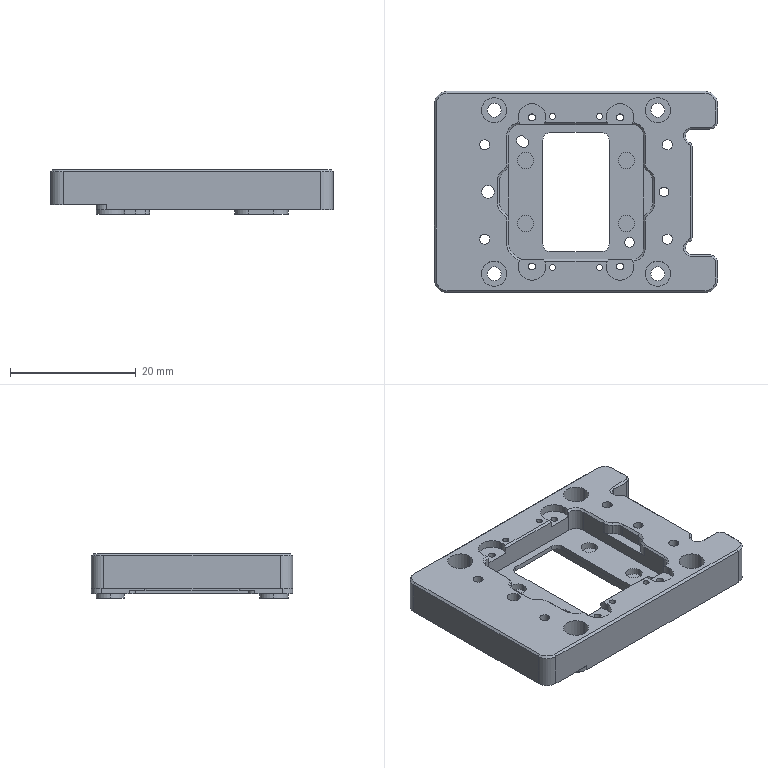NC program | NX | posted with a generic post | part box 45 x 32 x 7.05 mm
Lines 1920 to 2540 of 2540:
(PLANAR_MILL_COPY_COPY_COPY , TOOL : D6A45)
N3796 T01 M6
N3798 G54
N3800 G17 G0 G90 X13.45 Y12.567 S9500 M3
N3802 G43 Z30. H1
N3804 Z0.5
N3806 G94 G1 Z-0.5 F1250.
N3808 G3 X13.7 Y13. R0.5
N3810 X13. Y13.7 R0.7
N3812 X13.7 Y13. R-0.7
N3814 X13.45 Y13.433 R0.5
N3816 G1 Z0.5
N3818 G0 Z30.
N3820 X10.115 Y16.132
N3822 Z0.5
N3824 G1 Z-0.5
N3826 G3 X10.981 Y15.632 R1.
N3828 G1 X12.981
N3830 G2 X15.631 Y12.982 R2.65
N3832 X12.981 Y10.332 R2.65
N3834 G1 X8.981
N3836 G2 X7.064 Y11.153 R2.65
N3838 X7.096 Y11.735 R0.4
N3840 G3 X6.95 Y11.991 R0.15
N3842 G2 X6.432 Y12.259 R0.4
N3844 X8.981 Y15.632 R2.65
N3846 G1 X10.981
N3848 G3 X11.847 Y16.132 R1.
N3850 G1 Z0.5
N3852 G0 Z30.
N3854 X8.959 Y12.892
N3856 Z0.5
N3858 G1 Z-0.5
N3860 G3 X8.987 Y13.149 R0.5
N3862 X8.802 Y12.964 R0.185
N3864 X8.987 Y13.149 R-0.185
N3866 X9.014 Y12.892 R0.5
N3868 G1 Z0.5
N3870 G0 Z30.
N3872 X-12.567 Y13.45
N3874 Z0.5
N3876 G1 Z-0.5
N3878 G3 X-13. Y13.7 R0.5
N3880 X-13.7 Y13. R0.7
N3882 X-13. Y13.7 R-0.7
N3884 X-13.433 Y13.45 R0.5
N3886 G1 Z0.5
N3888 G0 Z30.
N3890 X-16.176 Y12.121
N3892 Z0.5
N3894 G1 Z-0.5
N3896 G3 X-15.676 Y12.987 R1.
N3898 G2 X-13.026 Y15.637 R2.65
N3900 X-15.676 Y12.987 R-2.65
N3902 G3 X-16.176 Y13.853 R1.
N3904 G1 Z0.5
N3906 G0 Z30.
N3908 X-13.433 Y-13.45
N3910 Z0.5
N3912 G1 Z-0.5
N3914 G3 X-13. Y-13.7 R0.5
N3916 X-12.3 Y-13. R0.7
N3918 X-13. Y-13.7 R-0.7
N3920 X-12.567 Y-13.45 R0.5
N3922 G1 Z0.5
N3924 G0 Z30.
N3926 X-10.159 Y-16.158
N3928 Z0.5
N3930 G1 Z-0.5
N3932 G3 X-11.025 Y-15.658 R1.
N3934 G1 X-13.025
N3936 G2 X-15.675 Y-13.008 R2.65
N3938 X-13.025 Y-10.358 R2.65
N3940 G1 X-9.025
N3942 G2 X-7.099 Y-11.187 R2.65
N3944 X-7.106 Y-11.744 R0.4
N3946 G3 X-6.963 Y-11.995 R0.15
N3948 G2 X-6.479 Y-12.272 R0.4
N3950 X-9.025 Y-15.658 R2.65
N3952 G1 X-11.025
N3954 G3 X-11.891 Y-16.158 R1.
N3956 G1 Z0.5
N3958 G0 Z30.
N3960 X-8.985 Y-12.956
N3962 Z0.5
N3964 G1 Z-0.5
N3966 G3 X-9.013 Y-13.213 R0.5
N3968 X-8.828 Y-13.028 R0.185
N3970 X-9.013 Y-13.213 R-0.185
N3972 X-9.04 Y-12.956 R0.5
N3974 G1 Z0.5
N3976 G0 Z30.
N3978 X13.842 Y-16.161
N3980 Z0.5
N3982 G1 Z-0.5
N3984 G3 X12.976 Y-15.661 R1.
N3986 G2 X10.326 Y-13.011 R2.65
N3988 X12.976 Y-15.661 R-2.65
N3990 G3 X12.11 Y-16.161 R1.
N3992 G1 Z0.5
N3994 G0 Z30.
N3996 X13.45 Y-13.433
N3998 Z0.5
N4000 G1 Z-0.5
N4002 G3 X13.7 Y-13. R0.5
N4004 X13. Y-12.3 R0.7
N4006 X13.7 Y-13. R-0.7
N4008 X13.45 Y-12.567 R0.5
N4010 G1 Z0.5
N4012 G0 Z30.
(PLANAR_MILL_COPY_COPY_COPY_COPY , TOOL : D6A45)
N4014 X-6.946 Y11.7
N4016 Z-0.2
N4018 G1 X-6.901 Z-0.212
N4020 X-6.85 Y11.751 Z-0.231
N4022 Y11.949 Z-0.285
N4024 X-6.901 Y12. Z-0.304
N4026 X-7.099 Z-0.357
N4028 X-7.15 Y11.949 Z-0.376
N4030 Y11.751 Z-0.43
N4032 X-7.099 Y11.7 Z-0.449
N4034 X-6.901 Z-0.502
N4036 X-6.85 Y11.751 Z-0.521
N4038 Y11.949 Z-0.575
N4040 X-6.901 Y12. Z-0.594
N4042 X-7.099 Z-0.647
N4044 X-7.15 Y11.949 Z-0.666
N4046 Y11.751 Z-0.719
N4048 X-7.099 Y11.7 Z-0.739
N4050 X-6.901 Z-0.792
N4052 X-6.85 Y11.751 Z-0.811
N4054 Y11.949 Z-0.864
N4056 X-6.901 Y12. Z-0.884
N4058 X-7.099 Z-0.937
N4060 X-7.15 Y11.949 Z-0.956
N4062 Y11.751 Z-1.009
N4064 X-7.099 Y11.7 Z-1.028
N4066 X-6.901 Z-1.082
N4068 X-6.85 Y11.751 Z-1.101
N4070 Y11.949 Z-1.154
N4072 X-6.901 Y12. Z-1.173
N4074 X-7. Z-1.2
N4076 G3 X-7.15 Y11.85 R0.15
N4078 X-7. Y12. R-0.15
N4080 X-6.891 Y11.765 R0.5
N4082 G1 Z-0.2
N4084 G0 Z30.
N4086 X-11.533 Y17.286
N4088 Z-0.2
N4090 G1 Z-1.2
N4092 Y17.268
N4094 G3 X-11.036 Y16.4 R1.
N4096 G1 X7.001
N4098 G3 X7.499 Y17.284 R1.
N4100 G1 Z-0.2
N4102 G0 Z30.
N4104 X11.433 Y-17.291
N4106 Z-0.2
N4108 G1 Z-1.2
N4110 Y-17.274
N4112 G3 X10.947 Y-16.4 R1.
N4114 G1 X-7.001
N4116 G3 X-7.488 Y-17.273 R1.
N4118 G1 X-14.561
N4120 G3 X-15.049 Y-16.4 R1.
N4122 G1 X-20.5
N4124 G2 X-22.9 Y-14. R2.4
N4126 G1 Y-11.214
N4128 G2 X-22.49 Y-10.224 R1.4
N4130 G1 X-22.276 Y-10.01
N4132 G2 X-21.286 Y-9.6 R1.4
N4134 G1 X-18.555
N4136 G3 X-19.552 Y-9.523 R1.
N4138 G1 Y-9.
N4140 Z-0.2
N4142 G0 Z30.
N4144 Y9.
N4146 Z-0.2
N4148 G1 Z-1.2
N4150 Y9.523
N4152 G3 X-18.555 Y9.6 R1.
N4154 G1 X-21.286
N4156 G2 X-22.276 Y10.01 R1.4
N4158 G1 X-22.49 Y10.224
N4160 G2 X-22.9 Y11.214 R1.4
N4162 G1 Y14.
N4164 G2 X-20.5 Y16.4 R2.4
N4166 G1 X-15.015
N4168 G3 X-14.518 Y17.286 R1.
N4170 G1 Z-0.2
N4172 G0 Z30.
N4174 X4.439 Y12.713
N4176 Z-0.2
N4178 G1 Z-1.2
N4180 X4.455 Y12.72
N4182 G3 X5.067 Y13.511 R1.
N4184 X4.25 Y13.8 R1.3
N4186 G1 X3.164
N4188 G2 X2.18 Y14.204 R1.4
N4190 G3 X-2.18 Y14.204 R3.1
N4192 G2 X-3.164 Y13.8 R1.4
N4194 G1 X-4.25
N4196 G3 X-5.55 Y12.5 R1.3
N4198 G1 Y-11.304
N4200 G3 X-4.679 Y-11.664 R1.
N4202 G1 X-4.503 Y-12.681
N4204 G3 X-5.103 Y-13.481 R1.
N4206 X-4.25 Y-13.8 R1.3
N4208 G1 X-3.164
N4210 G2 X-2.18 Y-14.204 R1.4
N4212 G3 X2.18 Y-14.204 R3.1
N4214 G2 X3.164 Y-13.8 R1.4
N4216 G1 X3.629
N4218 G3 X4.548 Y-13.419 R1.3
N4220 G1 X5.169 Y-12.798
N4222 G3 X5.55 Y-11.879 R1.3
N4224 G1 Y-10.917
N4226 G3 X4.668 Y-10.957 R1.
N4228 G1 Z-0.2
N4230 G0 Z30.
N4232 Y10.957
N4234 Z-0.2
N4236 G1 Z-1.2
N4238 G3 X5.55 Y10.917 R1.
N4240 G1 Y11.235
N4242 G3 X4.664 Y11.558 R1.
N4244 G1 Z-0.2
N4246 G0 Z30.
N4248 X-8.125 Y-7.876
N4250 Z-0.2
N4252 G1 Y-7.847 Z-0.208
N4254 X-8.226 Y-7.702 Z-0.255
N4256 X-8.369 Y-7.649 Z-0.296
N4258 X-8.226 Y-7.702 Z-0.337
N4260 X-8.125 Y-7.847 Z-0.384
N4262 Y-8.153 Z-0.466
N4264 X-8.347 Y-8.375 Z-0.55
N4266 X-8.522 Y-8.374 Z-0.597
N4268 X-8.347 Y-8.375 Z-0.644
N4270 X-8.125 Y-8.153 Z-0.728
N4272 Y-7.847 Z-0.81
N4274 X-8.226 Y-7.702 Z-0.858
N4276 X-8.369 Y-7.649 Z-0.899
N4278 X-8.226 Y-7.702 Z-0.94
N4280 X-8.125 Y-7.847 Z-0.987
N4282 Y-8.153 Z-1.069
N4284 X-8.347 Y-8.375 Z-1.153
N4286 X-8.522 Y-8.374 Z-1.2
N4288 G3 X-8.369 Y-7.649 R0.375
N4290 X-8.145 Y-8.096 R0.5
N4292 G1 Z-0.2
N4294 G0 Z30.
N4296 X6.946 Y-11.7
N4298 Z-0.2
N4300 G1 X6.901 Z-0.212
N4302 X6.85 Y-11.751 Z-0.231
N4304 Y-11.949 Z-0.285
N4306 X6.901 Y-12. Z-0.304
N4308 X7.099 Z-0.357
N4310 X7.15 Y-11.949 Z-0.376
N4312 Y-11.751 Z-0.43
N4314 X7.099 Y-11.7 Z-0.449
N4316 X6.901 Z-0.502
N4318 X6.85 Y-11.751 Z-0.521
N4320 Y-11.949 Z-0.575
N4322 X6.901 Y-12. Z-0.594
N4324 X7.099 Z-0.647
N4326 X7.15 Y-11.949 Z-0.666
N4328 Y-11.751 Z-0.719
N4330 X7.099 Y-11.7 Z-0.739
N4332 X6.901 Z-0.792
N4334 X6.85 Y-11.751 Z-0.811
N4336 Y-11.949 Z-0.864
N4338 X6.901 Y-12. Z-0.884
N4340 X7.099 Z-0.937
N4342 X7.15 Y-11.949 Z-0.956
N4344 Y-11.751 Z-1.009
N4346 X7.099 Y-11.7 Z-1.028
N4348 X6.901 Z-1.082
N4350 X6.85 Y-11.751 Z-1.101
N4352 Y-11.949 Z-1.154
N4354 X6.901 Y-12. Z-1.173
N4356 X7. Z-1.2
N4358 G3 X7.15 Y-11.85 R0.15
N4360 X7. Y-12. R-0.15
N4362 X6.891 Y-11.765 R0.5
N4364 G1 Z-0.2
N4366 G0 Z30.
(PLANAR_MILL_COPY_COPY_COPY_COPY_COPY , TOOL : D6A45)
N4368 X16.459 Y17.901
N4370 Z-1.5
N4372 G1 Z-2.5
N4374 X16.453 Y17.885
N4376 G3 X16.625 Y16.9 R1.
N4378 G1 X20.5
N4380 G2 X23.4 Y14. R2.9
N4382 G1 Y-14.
N4384 G2 X20.5 Y-16.9 R2.9
N4386 G1 X16.625
N4388 G3 X16.459 Y-17.901 R1.
N4390 G1 Z-1.5
N4392 G0 Z30.
(PLANAR_MILL_COPY_COPY_COPY_COPY_COPY_COPY , TOOL : D6A45)
N4394 X-20.071 Y-7.4
N4396 Z-1.2
N4398 G1 Z-2.2
N4400 X-20.013 Y-7.5
N4402 G3 X-19.147 Y-8. R1.
N4404 G2 X-19.4 Y-7.053 R1.9
N4406 G1 Y7.053
N4408 G2 X-19.147 Y8. R1.9
N4410 G3 X-20.013 Y7.5 R1.
N4412 G1 X-20.071 Y7.4
N4414 Z-1.2
N4416 G0 Z30.
N4418 X4.069 Y-7.842
N4420 Z-1.2
N4422 G1 Z-2.2
N4424 G3 X5.05 Y-7.678 R1.
N4426 G1 Y7.678
N4428 G3 X4.069 Y7.842 R1.
N4430 G1 Z-1.2
N4432 G0 Z30.
N4434 M5
(ZLEVEL_PROFILE_2_COPY , TOOL : R0.75)
N4436 T15 M6
N4438 G54
N4440 G17 G0 G90 X18.742 Y2.918 S9500 M3
N4442 G43 Z30. H15
N4444 Z1.5
N4446 G94 G1 Z-1.61 F500.
N4448 X19.467 F1250.
N4450 Y3.305
N4452 G3 X19.362 Y3.678 R0.61
N4454 X18.758 Y3.563 R0.335
N4456 G1 X18.749 Y3.524
N4458 X18.709 Y3.433
N4460 G3 X18.103 Y3.614 R0.343
N4462 X18.017 Y3.376 R0.372
N4464 G1 Y2.918
N4466 X18.742
N4468 Z1.39
N4470 G0 Z30.
N4472 X18.388 Y3.01
N4474 Z1.5
N4476 G1 Z-1.61 F500.
N4478 X18.114 F1250.
N4480 X18.087 Y3.009
N4482 X18.089 Y3.035
N4484 Y3.344
N4486 G2 X18.686 Y3.456 R0.309
N4488 G1 Y3.035
N4490 X18.661 Y3.01
N4492 X18.388
N4494 Z1.39
N4496 G0 Z30.
N4498 X19.063
N4500 Z1.5
N4502 G1 Z-1.61 F500.
N4504 X18.783 F1250.
N4506 X18.758 Y3.02
N4508 Y3.342
N4510 G2 X18.848 Y3.614 R0.456
N4512 X19.378 Y3.466 R0.295
N4514 G1 X19.396 Y3.285
N4516 Y3.035
N4518 X19.397 Y3.009
N4520 X19.371 Y3.01
N4522 X19.063
N4524 Z1.39
N4526 G0 Z30.
N4528 X18.694 Y2.199
N4530 Z1.5
N4532 G1 Z-1.61 F500.
N4534 X18.017 F1250.
N4536 Y2.103
N4538 X18.059 Y2.048
N4540 X18.249 Y1.763
N4542 X18.311
N4544 X18.113 Y2.069
N4546 X18.134 Y2.107
N4548 X19.371
N4550 X19.397 Y2.109
N4552 X19.396 Y2.082
N4554 Y1.722
N4556 X19.467
N4558 Y2.524
N4560 X19.396
N4562 Y2.224
N4564 X19.397 Y2.198
N4566 X19.371 Y2.199
N4568 X18.694
N4570 Z1.39
N4572 G0 Z30.
N4574 X18.669 Y0.758
N4576 Z1.5
N4578 G1 Z-1.61 F500.
N4580 X18.7 Y0.809 F1250.
N4582 X18.712
N4584 G3 X19.488 Y0.956 R0.395
N4586 X18.711 Y1.107 R0.396
N4588 G1 X18.692 Y1.106
N4590 G3 X18.244 Y1.347 R0.36
N4592 X18.002 Y0.901 R0.36
N4594 X18.639 Y0.706 R0.346
N4596 G1 X18.669 Y0.758
N4598 Z1.39
N4600 G0 Z30.
N4602 X18.653 Y0.957
N4604 Z1.5
N4606 G1 Z-1.61 F500.
N4608 X18.651 Y0.847 F1250.
N4610 X18.639 Y0.803
N4612 X18.677 Y0.788
N4614 X18.597 Y0.737
N4616 X18.585 Y0.724
N4618 G2 X18.072 Y1.011 R0.304
N4620 X18.622 Y1.145 R0.299
N4622 G1 X18.674 Y1.124
N4624 X18.639 Y1.11
N4626 X18.654 Y1.065
N4628 X18.653 Y0.957
N4630 Z1.39
N4632 G0 Z30.
N4634 X18.793 Y1.18
N4636 Z1.5
N4638 G1 Z-1.61 F500.
N4640 X18.831 Y1.229 F1250.
N4642 G2 X18.872 Y0.656 R-0.361
N4644 G3 X18.724 Y0.803 R0.949
N4646 X18.728 Y1.13 R0.599
N4648 G1 X18.735 Y1.116
N4650 X18.75 Y1.117
N4652 X18.756 Y1.131
N4654 X18.793 Y1.18
N4656 Z1.39
N4658 G0 Z30.
N4660 X18.694 Y-0.112
N4662 Z1.5
N4664 G1 Z-1.61 F500.
N4666 X18.017 F1250.
N4668 Y-0.2
N4670 X18.249 Y-0.548
N4672 X18.311
N4674 X18.113 Y-0.242
N4676 X18.134 Y-0.203
N4678 X19.371
N4680 X19.397 Y-0.202
N4682 X19.396 Y-0.228
N4684 Y-0.589
N4686 X19.467
N4688 Y0.213
N4690 X19.396
N4692 Y-0.087
N4694 X19.397 Y-0.113
N4696 X19.371 Y-0.112
N4698 X18.694
N4700 Z1.39
N4702 G0 Z30.
N4704 X18.729 Y-1.633
N4706 Z1.5
N4708 G1 Z-1.61 F500.
N4710 X18.767 Y-1.667 F1250.
N4712 X18.768 Y-1.688
N4714 G2 X18.207 Y-1.561 R0.844
N4716 X18.247 Y-1.031 R0.302
N4718 G1 X18.228 Y-0.95
N4720 G3 X18.209 Y-1.667 R0.398
N4722 X19.202 Y-1.716 R1.387
N4724 X19.067 Y-0.908 R0.414
N4726 X18.692 Y-1.6 R0.407
N4728 G1 X18.729 Y-1.633
N4730 Z1.39
N4732 G0 Z30.
N4734 X19.412 Y-1.327
N4736 Z1.5
N4738 G1 Z-1.61 F500.
N4740 G2 X19.067 Y-1.665 R0.338 F1250.
N4742 X19.013 Y-0.994 R-0.342
N4744 X19.412 Y-1.327 R0.338
N4746 G1 Z1.39
N4748 G0 Z30.
N4750 X17.999 Y-2.492
N4752 Z1.5
N4754 G1 Z-1.61 F500.
N4756 G3 X18.287 Y-2.891 R0.414 F1250.
N4758 X19.227 Y-2.88 R1.487
N4760 X19.249 Y-2.131 R0.405
N4762 X18.296 Y-2.1 R1.518
N4764 X17.999 Y-2.492 R0.414
N4766 G1 Z1.39
N4768 G0 Z30.
N4770 X18.774 Y-2.127
N4772 Z1.5
N4774 G1 Z-1.61 F500.
N4776 G2 X19.227 Y-2.207 R1.564 F1250.
N4778 X19.164 Y-2.814 R0.321
N4780 X18.317 Y-2.816 R1.645
N4782 X18.317 Y-2.181 R0.326
N4784 X18.774 Y-2.127 R1.564
N4786 G1 Z1.39
N4788 G0 Z30.
N4790 X18.344 Y-4.06
N4792 Z1.5
N4794 G1 Z-1.61 F500.
N4796 X18.371 Y-4.065 F1250.
N4798 G3 X19.209 Y-4.043 R1.425
N4800 X19.227 Y-3.279 R0.406
N4802 X18.307 Y-3.251 R1.525
N4804 X18.317 Y-4.055 R0.413
N4806 G1 X18.344 Y-4.06
N4808 Z1.39
N4810 G0 Z30.
N4812 X18.749 Y-4.025
N4814 Z1.5
N4816 G1 Z-1.61 F500.
N4818 G2 X18.317 Y-3.971 R1.672 F1250.
N4820 X18.317 Y-3.337 R0.326
N4822 X19.208 Y-3.368 R1.384
N4824 X19.18 Y-3.966 R0.315
N4826 X18.749 Y-4.025 R1.672
N4828 G1 Z1.39
N4830 G0 Z30.
N4832 X19.482 Y-4.827
N4834 Z1.5
N4836 G1 Z-1.61 F500.
N4838 G3 X19.218 Y-4.436 R0.407 F1250.
N4840 X18.21 Y-4.444 R1.409
N4842 X18.286 Y-5.207 R0.417
N4844 X19.2 Y-5.204 R1.509
N4846 X19.482 Y-4.827 R0.407
N4848 G1 Z1.39
N4850 G0 Z30.
N4852 X18.774 Y-4.437
N4854 Z1.5
N4856 G1 Z-1.61 F500.
N4858 G2 X19.227 Y-4.518 R1.55 F1250.
N4860 X19.12 Y-5.142 R0.329
N4862 X18.317 Y-5.127 R1.82
N4864 X18.317 Y-4.493 R0.326
N4866 X18.774 Y-4.437 R1.55
N4868 G1 Z1.39
N4870 G0 Z30.
N4872 X18.981 Y-5.945
N4874 Z1.5
N4876 G1 Z-1.61 F500.
N4878 Y-5.666 F1250.
N4880 X18.909
N4882 Y-6.224
N4884 X18.981
N4886 Y-5.945
N4888 Z1.39
N4890 G0 Z30.
N4892 Y-7.083
N4894 Z1.5
N4896 G1 Z-1.61 F500.
N4898 X18.639 Y-6.751 F1250.
N4900 G3 X18.002 Y-7.075 R0.382
N4902 X18.319 Y-7.475 R0.374
N4904 G1 X18.33 Y-7.39
N4906 G2 X18.532 Y-6.781 R-0.324
N4908 X18.928 Y-7.13 R1.273
N4910 G3 X19.402 Y-7.501 R1.44
N4912 G1 X19.467
N4914 Y-6.639
N4916 X19.396
N4918 Y-7.384
N4920 X19.391 Y-7.417
N4922 X19.358 Y-7.425
N4924 X19.338 Y-7.398
N4926 X19.227 Y-7.322
N4928 X18.981 Y-7.083
N4930 Z1.39
N4932 G0 Z30.
N4934 X19.487 Y-8.217
N4936 Z1.5
N4938 G1 Z-1.61 F500.
N4940 G3 X19.22 Y-7.837 R0.403 F1250.
N4942 X18.285 Y-7.824 R1.444
N4944 X18.284 Y-8.607 R0.412
N4946 X19.218 Y-8.596 R1.45
N4948 X19.487 Y-8.217 R0.403
N4950 G1 Z1.39
N4952 G0 Z30.
N4954 X18.761 Y-8.588
N4956 Z1.5
N4958 G1 Z-1.61 F500.
N4960 G2 X18.294 Y-8.517 R1.495 F1250.
N4962 X18.302 Y-7.902 R0.322
N4964 X19.227 Y-7.924 R1.538
N4966 X19.227 Y-8.51 R0.32
N4968 X18.761 Y-8.588 R1.495
N4970 G1 Z1.39
N4972 G0 Z30.
N4974 X18.017 Y-9.37
N4976 Z1.5
N4978 G1 Z-1.61 F500.
N4980 Y-9.812 F1250.
N4982 X18.089
N4984 Y-9.046
N4986 X18.189 Y-9.036
N4988 X18.262 Y-9.106
N4990 G3 X19.467 Y-9.524 R2.52
N4992 G1 Y-9.436
N4994 G2 X18.103 Y-8.929 R2.681
N4996 G1 X18.017
N4998 Y-9.37
N5000 Z1.39
N5002 G0 Z30.
N5004 M5
N5006 M2